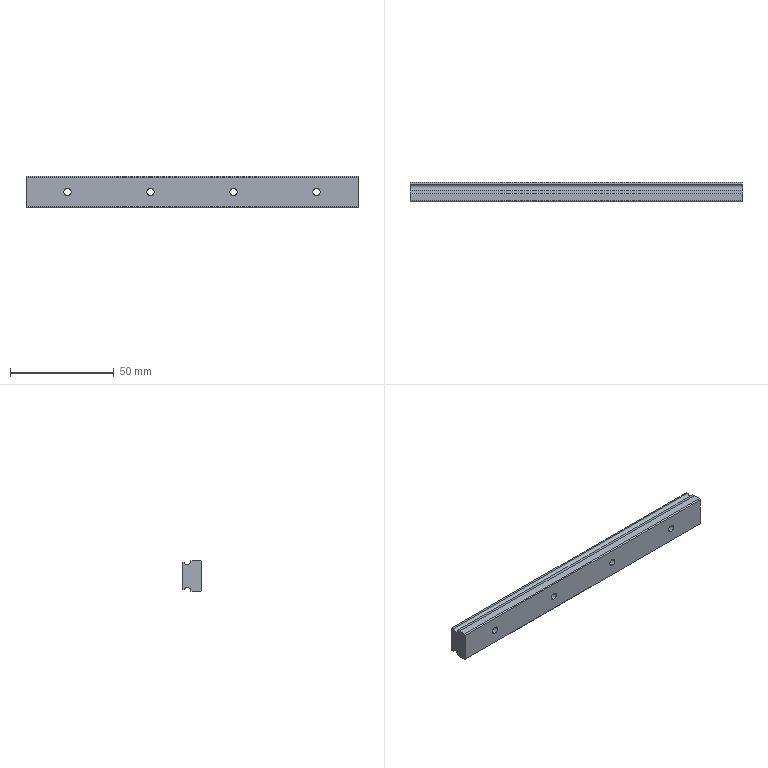Part | STEP file | RSR15M1V160201 Track^SRS15MUU-160LM-G20_Pay-off clamp assembly | 1 solid | 35 faces | box 160 x 9.5 x 15 mm | volume 20064 mm3 | cylinder 19 | plane 16 | commonest cylinder face diameters 3.5 x8 6 x8 3.18 x3